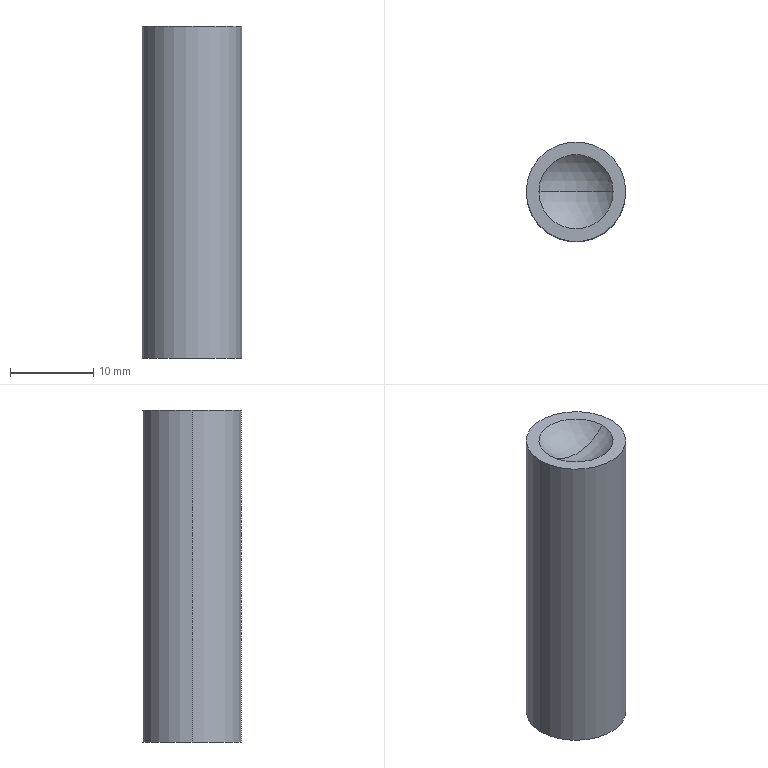Part | SolidWorks | features Extrusion 1, RevCut 1 | 1 solid | 6 faces | box 12 x 12 x 40 mm | volume 4457 mm3 | sphere 2 | cylinder 2 | plane 2 | commonest cylinder face diameters 12 x2
STEP:
#1=CARTESIAN_POINT('',(0.,0.,38.));
#2=VERTEX_POINT('',#1);
#3=CARTESIAN_POINT('',(-4.472,0.,40.));
#4=VERTEX_POINT('',#3);
#5=CARTESIAN_POINT('',(0.,0.,44.));
#6=DIRECTION('',(0.,1.,0.));
#7=DIRECTION('',(0.,0.,1.));
#8=AXIS2_PLACEMENT_3D('',#5,#6,#7);
#9=CIRCLE('',#8,6.);
#10=EDGE_CURVE('',#2,#4,#9,.T.);
#11=ORIENTED_EDGE('',*,*,#10,.F.);
#12=CARTESIAN_POINT('',(4.472,0.,40.));
#13=VERTEX_POINT('',#12);
#14=CARTESIAN_POINT('',(0.,0.,44.));
#15=DIRECTION('',(0.,-1.,0.));
#16=DIRECTION('',(1.,0.,0.));
#17=AXIS2_PLACEMENT_3D('',#14,#15,#16);
#18=CIRCLE('',#17,6.);
#19=EDGE_CURVE('',#2,#13,#18,.T.);
#20=ORIENTED_EDGE('',*,*,#19,.T.);
#21=CARTESIAN_POINT('',(0.,0.,40.));
#22=DIRECTION('',(0.,0.,-1.));
#23=DIRECTION('',(1.,0.,0.));
#24=AXIS2_PLACEMENT_3D('',#21,#22,#23);
#25=CIRCLE('',#24,4.472);
#26=EDGE_CURVE('',#4,#13,#25,.T.);
#27=ORIENTED_EDGE('',*,*,#26,.F.);
#28=EDGE_LOOP('',(#11,#20,#27));
#29=FACE_OUTER_BOUND('',#28,.T.);
#30=CARTESIAN_POINT('',(0.,0.,44.));
#31=DIRECTION('',(0.,-1.,0.));
#32=DIRECTION('',(-1.,0.,0.));
#33=AXIS2_PLACEMENT_3D('',#30,#31,#32);
#34=SPHERICAL_SURFACE('',#33,6.);
#35=ADVANCED_FACE('',(#29),#34,.F.);
#36=CARTESIAN_POINT('',(6.,0.,40.));
#37=VERTEX_POINT('',#36);
#38=CARTESIAN_POINT('',(-6.,0.,40.));
#39=VERTEX_POINT('',#38);
#40=CARTESIAN_POINT('',(0.,0.,40.));
#41=DIRECTION('',(0.,0.,1.));
#42=DIRECTION('',(1.,0.,0.));
#43=AXIS2_PLACEMENT_3D('',#40,#41,#42);
#44=CIRCLE('',#43,6.);
#45=EDGE_CURVE('',#37,#39,#44,.T.);
#46=ORIENTED_EDGE('',*,*,#45,.F.);
#47=CARTESIAN_POINT('',(6.,0.,0.));
#48=VERTEX_POINT('',#47);
#49=CARTESIAN_POINT('',(6.,0.,40.));
#50=DIRECTION('',(0.,0.,-1.));
#51=VECTOR('',#50,1000.);
#52=LINE('',#49,#51);
#53=EDGE_CURVE('',#37,#48,#52,.T.);
#54=ORIENTED_EDGE('',*,*,#53,.T.);
#55=CARTESIAN_POINT('',(-6.,0.,0.));
#56=VERTEX_POINT('',#55);
#57=CARTESIAN_POINT('',(0.,0.,0.));
#58=DIRECTION('',(0.,0.,1.));
#59=DIRECTION('',(1.,0.,0.));
#60=AXIS2_PLACEMENT_3D('',#57,#58,#59);
#61=CIRCLE('',#60,6.);
#62=EDGE_CURVE('',#48,#56,#61,.T.);
#63=ORIENTED_EDGE('',*,*,#62,.T.);
#64=CARTESIAN_POINT('',(-6.,0.,40.));
#65=DIRECTION('',(0.,0.,-1.));
#66=VECTOR('',#65,1000.);
#67=LINE('',#64,#66);
#68=EDGE_CURVE('',#39,#56,#67,.T.);
#69=ORIENTED_EDGE('',*,*,#68,.F.);
#70=EDGE_LOOP('',(#46,#54,#63,#69));
#71=FACE_OUTER_BOUND('',#70,.T.);
#72=CARTESIAN_POINT('',(0.,0.,40.));
#73=DIRECTION('',(0.,0.,-1.));
#74=DIRECTION('',(-1.,0.,0.));
#75=AXIS2_PLACEMENT_3D('',#72,#73,#74);
#76=CYLINDRICAL_SURFACE('',#75,6.);
#77=ADVANCED_FACE('',(#71),#76,.T.);
#78=ORIENTED_EDGE('',*,*,#53,.F.);
#79=CARTESIAN_POINT('',(0.,0.,40.));
#80=DIRECTION('',(0.,0.,1.));
#81=DIRECTION('',(1.,0.,0.));
#82=AXIS2_PLACEMENT_3D('',#79,#80,#81);
#83=CIRCLE('',#82,6.);
#84=EDGE_CURVE('',#39,#37,#83,.T.);
#85=ORIENTED_EDGE('',*,*,#84,.F.);
#86=ORIENTED_EDGE('',*,*,#68,.T.);
#87=CARTESIAN_POINT('',(0.,0.,0.));
#88=DIRECTION('',(0.,0.,1.));
#89=DIRECTION('',(1.,0.,0.));
#90=AXIS2_PLACEMENT_3D('',#87,#88,#89);
#91=CIRCLE('',#90,6.);
#92=EDGE_CURVE('',#56,#48,#91,.T.);
#93=ORIENTED_EDGE('',*,*,#92,.T.);
#94=EDGE_LOOP('',(#78,#85,#86,#93));
#95=FACE_OUTER_BOUND('',#94,.T.);
#96=CARTESIAN_POINT('',(0.,0.,40.));
#97=DIRECTION('',(0.,0.,-1.));
#98=DIRECTION('',(-1.,0.,0.));
#99=AXIS2_PLACEMENT_3D('',#96,#97,#98);
#100=CYLINDRICAL_SURFACE('',#99,6.);
#101=ADVANCED_FACE('',(#95),#100,.T.);
#102=ORIENTED_EDGE('',*,*,#26,.T.);
#103=CARTESIAN_POINT('',(0.,0.,40.));
#104=DIRECTION('',(0.,0.,-1.));
#105=DIRECTION('',(1.,0.,0.));
#106=AXIS2_PLACEMENT_3D('',#103,#104,#105);
#107=CIRCLE('',#106,4.472);
#108=EDGE_CURVE('',#13,#4,#107,.T.);
#109=ORIENTED_EDGE('',*,*,#108,.T.);
#110=EDGE_LOOP('',(#102,#109));
#111=FACE_BOUND('',#110,.T.);
#112=ORIENTED_EDGE('',*,*,#84,.T.);
#113=ORIENTED_EDGE('',*,*,#45,.T.);
#114=EDGE_LOOP('',(#112,#113));
#115=FACE_OUTER_BOUND('',#114,.T.);
#116=CARTESIAN_POINT('',(0.,0.,40.));
#117=DIRECTION('',(0.,0.,1.));
#118=DIRECTION('',(1.,0.,0.));
#119=AXIS2_PLACEMENT_3D('',#116,#117,#118);
#120=PLANE('',#119);
#121=ADVANCED_FACE('',(#111,#115),#120,.T.);
#122=ORIENTED_EDGE('',*,*,#92,.F.);
#123=ORIENTED_EDGE('',*,*,#62,.F.);
#124=EDGE_LOOP('',(#122,#123));
#125=FACE_OUTER_BOUND('',#124,.T.);
#126=CARTESIAN_POINT('',(0.,0.,0.));
#127=DIRECTION('',(0.,0.,1.));
#128=DIRECTION('',(1.,0.,0.));
#129=AXIS2_PLACEMENT_3D('',#126,#127,#128);
#130=PLANE('',#129);
#131=ADVANCED_FACE('',(#125),#130,.F.);
#132=ORIENTED_EDGE('',*,*,#19,.F.);
#133=ORIENTED_EDGE('',*,*,#10,.T.);
#134=ORIENTED_EDGE('',*,*,#108,.F.);
#135=EDGE_LOOP('',(#132,#133,#134));
#136=FACE_OUTER_BOUND('',#135,.T.);
#137=CARTESIAN_POINT('',(0.,0.,44.));
#138=DIRECTION('',(0.,-1.,0.));
#139=DIRECTION('',(-1.,0.,0.));
#140=AXIS2_PLACEMENT_3D('',#137,#138,#139);
#141=SPHERICAL_SURFACE('',#140,6.);
#142=ADVANCED_FACE('',(#136),#141,.F.);
#143=CLOSED_SHELL('',(#35,#77,#101,#121,#131,#142));
#144=MANIFOLD_SOLID_BREP('',#143);
#145=CARTESIAN_POINT('',(0.,0.,0.));
#146=DIRECTION('',(0.,0.,1.));
#147=DIRECTION('',(1.,0.,0.));
#148=AXIS2_PLACEMENT_3D('',#145,#146,#147);
#149=(LENGTH_UNIT()NAMED_UNIT(*)SI_UNIT(.MILLI.,.METRE.));
#150=UNCERTAINTY_MEASURE_WITH_UNIT(LENGTH_MEASURE(0.00001),#149,'','');
#151=(NAMED_UNIT(*)PLANE_ANGLE_UNIT()SI_UNIT($,.RADIAN.));
#152=(NAMED_UNIT(*)SI_UNIT($,.STERADIAN.)SOLID_ANGLE_UNIT());
#153=(GEOMETRIC_REPRESENTATION_CONTEXT(3)GLOBAL_UNCERTAINTY_ASSIGNED_CONTEXT((#150))GLOBAL_UNIT_ASSIGNED_CONTEXT((#149,#151,#152))REPRESENTATION_CONTEXT('',''));
#154=ADVANCED_BREP_SHAPE_REPRESENTATION('',(#144,#148),#153);